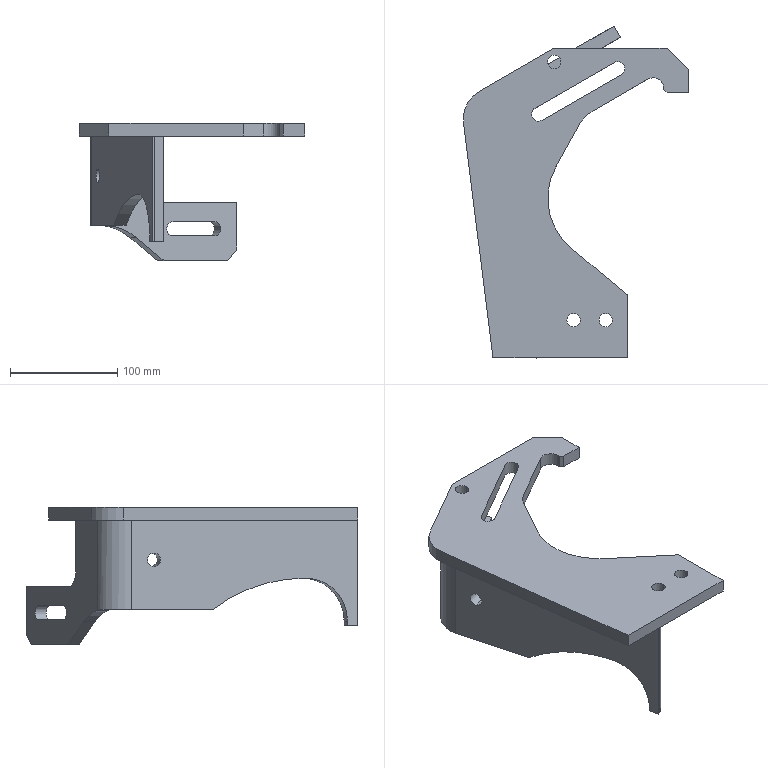Part | SolidWorks | features BaseBody 2 | 2 solids | 62 faces | box 209.597 x 308.937 x 128 mm | volume 664843 mm3 | plane 38 | cylinder 23 | spline 1 | commonest cylinder face diameters 12.5 x8 13 x3 13.3 x2 60 x2 120 x2 20 x1